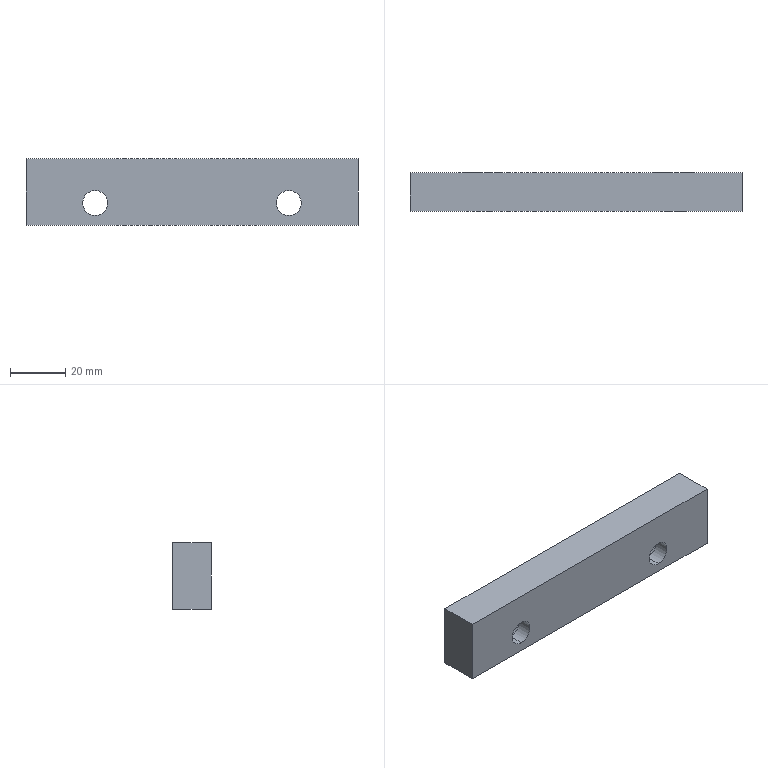Part | STEP file | 1 solid | 16 faces | box 120 x 14 x 24 mm | volume 36593 mm3 | cylinder 8 | plane 8 | commonest cylinder face diameters 9 x4 15 x4
STEP:
#1=CARTESIAN_POINT('',(0.,0.,0.));
#2=DIRECTION('',(0.,0.,1.));
#3=DIRECTION('',(1.,0.,0.));
#4=AXIS2_PLACEMENT_3D('',#1,#2,#3);
#5=CARTESIAN_POINT('',(-35.,5.4,15.5));
#6=VERTEX_POINT('',#5);
#7=CARTESIAN_POINT('',(-35.,14.,15.5));
#8=VERTEX_POINT('',#7);
#9=CARTESIAN_POINT('',(-35.,14.,15.5));
#10=DIRECTION('',(0.,1.,0.));
#11=VECTOR('',#10,1.);
#12=LINE('',#9,#11);
#13=CARTESIAN_POINT('',(-35.,14.,8.));
#14=DIRECTION('',(0.,1.,0.));
#15=DIRECTION('',(0.,0.,1.));
#16=AXIS2_PLACEMENT_3D('',#13,#14,#15);
#17=CYLINDRICAL_SURFACE('',#16,7.5);
#18=CARTESIAN_POINT('',(6.283,0.));
#19=DIRECTION('',(0.,1.));
#20=VECTOR('',#19,1.);
#21=LINE('',#18,#20);
#22=(GEOMETRIC_REPRESENTATION_CONTEXT(2)PARAMETRIC_REPRESENTATION_CONTEXT()REPRESENTATION_CONTEXT('',''));
#23=DEFINITIONAL_REPRESENTATION('',(#21),#22);
#24=PCURVE('',#17,#23);
#25=CARTESIAN_POINT('',(-35.,14.,8.));
#26=DIRECTION('',(0.,1.,0.));
#27=DIRECTION('',(0.,0.,1.));
#28=AXIS2_PLACEMENT_3D('',#25,#26,#27);
#29=CYLINDRICAL_SURFACE('',#28,7.5);
#30=CARTESIAN_POINT('',(0.,0.));
#31=DIRECTION('',(0.,1.));
#32=VECTOR('',#31,1.);
#33=LINE('',#30,#32);
#34=(GEOMETRIC_REPRESENTATION_CONTEXT(2)PARAMETRIC_REPRESENTATION_CONTEXT()REPRESENTATION_CONTEXT('',''));
#35=DEFINITIONAL_REPRESENTATION('',(#33),#34);
#36=PCURVE('',#29,#35);
#37=SURFACE_CURVE('',#12,(#24,#36),.PCURVE_S1.);
#38=EDGE_CURVE('',#6,#8,#37,.T.);
#39=ORIENTED_EDGE('',*,*,#38,.T.);
#40=CARTESIAN_POINT('',(-35.,14.,0.5));
#41=VERTEX_POINT('',#40);
#42=CARTESIAN_POINT('',(-35.,14.,8.));
#43=DIRECTION('',(0.,1.,0.));
#44=DIRECTION('',(0.,0.,1.));
#45=AXIS2_PLACEMENT_3D('',#42,#43,#44);
#46=CIRCLE('',#45,7.5);
#47=CARTESIAN_POINT('',(0.,0.));
#48=DIRECTION('',(1.,0.));
#49=VECTOR('',#48,1.);
#50=LINE('',#47,#49);
#51=(GEOMETRIC_REPRESENTATION_CONTEXT(2)PARAMETRIC_REPRESENTATION_CONTEXT()REPRESENTATION_CONTEXT('',''));
#52=DEFINITIONAL_REPRESENTATION('',(#50),#51);
#53=PCURVE('',#17,#52);
#54=CARTESIAN_POINT('',(0.,14.,0.));
#55=DIRECTION('',(0.,1.,0.));
#56=DIRECTION('',(0.,0.,1.));
#57=AXIS2_PLACEMENT_3D('',#54,#55,#56);
#58=PLANE('',#57);
#59=CARTESIAN_POINT('',(8.,-35.));
#60=DIRECTION('',(1.,0.));
#61=AXIS2_PLACEMENT_2D('',#59,#60);
#62=CIRCLE('',#61,7.5);
#63=(GEOMETRIC_REPRESENTATION_CONTEXT(2)PARAMETRIC_REPRESENTATION_CONTEXT()REPRESENTATION_CONTEXT('',''));
#64=DEFINITIONAL_REPRESENTATION('',(#62),#63);
#65=PCURVE('',#58,#64);
#66=SURFACE_CURVE('',#46,(#53,#65),.PCURVE_S1.);
#67=EDGE_CURVE('',#41,#8,#66,.T.);
#68=ORIENTED_EDGE('',*,*,#67,.F.);
#69=CARTESIAN_POINT('',(-35.,5.4,0.5));
#70=VERTEX_POINT('',#69);
#71=CARTESIAN_POINT('',(-35.,14.,0.5));
#72=DIRECTION('',(0.,1.,0.));
#73=VECTOR('',#72,1.);
#74=LINE('',#71,#73);
#75=CARTESIAN_POINT('',(3.142,0.));
#76=DIRECTION('',(0.,1.));
#77=VECTOR('',#76,1.);
#78=LINE('',#75,#77);
#79=(GEOMETRIC_REPRESENTATION_CONTEXT(2)PARAMETRIC_REPRESENTATION_CONTEXT()REPRESENTATION_CONTEXT('',''));
#80=DEFINITIONAL_REPRESENTATION('',(#78),#79);
#81=PCURVE('',#17,#80);
#82=CARTESIAN_POINT('',(3.142,0.));
#83=DIRECTION('',(0.,1.));
#84=VECTOR('',#83,1.);
#85=LINE('',#82,#84);
#86=(GEOMETRIC_REPRESENTATION_CONTEXT(2)PARAMETRIC_REPRESENTATION_CONTEXT()REPRESENTATION_CONTEXT('',''));
#87=DEFINITIONAL_REPRESENTATION('',(#85),#86);
#88=PCURVE('',#29,#87);
#89=SURFACE_CURVE('',#74,(#81,#88),.PCURVE_S1.);
#90=EDGE_CURVE('',#70,#41,#89,.T.);
#91=ORIENTED_EDGE('',*,*,#90,.F.);
#92=CARTESIAN_POINT('',(-35.,5.4,8.));
#93=DIRECTION('',(0.,1.,0.));
#94=DIRECTION('',(0.,0.,1.));
#95=AXIS2_PLACEMENT_3D('',#92,#93,#94);
#96=CIRCLE('',#95,7.5);
#97=CARTESIAN_POINT('',(0.,-8.6));
#98=DIRECTION('',(1.,0.));
#99=VECTOR('',#98,1.);
#100=LINE('',#97,#99);
#101=(GEOMETRIC_REPRESENTATION_CONTEXT(2)PARAMETRIC_REPRESENTATION_CONTEXT()REPRESENTATION_CONTEXT('',''));
#102=DEFINITIONAL_REPRESENTATION('',(#100),#101);
#103=PCURVE('',#17,#102);
#104=CARTESIAN_POINT('',(-30.5,5.4,8.));
#105=DIRECTION('',(0.,-1.,0.));
#106=DIRECTION('',(0.,0.,-1.));
#107=AXIS2_PLACEMENT_3D('',#104,#105,#106);
#108=PLANE('',#107);
#109=CARTESIAN_POINT('',(-7.5,-4.5));
#110=CARTESIAN_POINT('',(-7.5,8.49));
#111=CARTESIAN_POINT('',(3.75,1.995));
#112=CARTESIAN_POINT('',(15.,-4.5));
#113=CARTESIAN_POINT('',(3.75,-10.995));
#114=CARTESIAN_POINT('',(-7.5,-17.49));
#115=CARTESIAN_POINT('',(-7.5,-4.5));
#116=(BOUNDED_CURVE()B_SPLINE_CURVE(2,(#109,#110,#111,#112,#113,#114,#115),.UNSPECIFIED.,.T.,.F.)B_SPLINE_CURVE_WITH_KNOTS((1,2,2,2,2,1),(-2.094,0.,2.094,4.189,6.283,8.378),.UNSPECIFIED.)CURVE()GEOMETRIC_REPRESENTATION_ITEM()RATIONAL_B_SPLINE_CURVE((1.,0.5,1.,0.5,1.,0.5,1.))REPRESENTATION_ITEM(''));
#117=(GEOMETRIC_REPRESENTATION_CONTEXT(2)PARAMETRIC_REPRESENTATION_CONTEXT()REPRESENTATION_CONTEXT('',''));
#118=DEFINITIONAL_REPRESENTATION('',(#116),#117);
#119=PCURVE('',#108,#118);
#120=SURFACE_CURVE('',#96,(#103,#119),.PCURVE_S1.);
#121=EDGE_CURVE('',#70,#6,#120,.T.);
#122=ORIENTED_EDGE('',*,*,#121,.T.);
#123=EDGE_LOOP('',(#39,#68,#91,#122));
#124=FACE_BOUND('',#123,.F.);
#125=ADVANCED_FACE('',(#124),#17,.F.);
#126=CARTESIAN_POINT('',(-35.,0.,12.5));
#127=VERTEX_POINT('',#126);
#128=CARTESIAN_POINT('',(-35.,5.4,12.5));
#129=VERTEX_POINT('',#128);
#130=CARTESIAN_POINT('',(-35.,14.,12.5));
#131=DIRECTION('',(0.,1.,0.));
#132=VECTOR('',#131,1.);
#133=LINE('',#130,#132);
#134=CARTESIAN_POINT('',(-35.,14.,8.));
#135=DIRECTION('',(0.,1.,0.));
#136=DIRECTION('',(0.,0.,1.));
#137=AXIS2_PLACEMENT_3D('',#134,#135,#136);
#138=CYLINDRICAL_SURFACE('',#137,4.5);
#139=CARTESIAN_POINT('',(6.283,0.));
#140=DIRECTION('',(0.,1.));
#141=VECTOR('',#140,1.);
#142=LINE('',#139,#141);
#143=(GEOMETRIC_REPRESENTATION_CONTEXT(2)PARAMETRIC_REPRESENTATION_CONTEXT()REPRESENTATION_CONTEXT('',''));
#144=DEFINITIONAL_REPRESENTATION('',(#142),#143);
#145=PCURVE('',#138,#144);
#146=CARTESIAN_POINT('',(-35.,14.,8.));
#147=DIRECTION('',(0.,1.,0.));
#148=DIRECTION('',(0.,0.,1.));
#149=AXIS2_PLACEMENT_3D('',#146,#147,#148);
#150=CYLINDRICAL_SURFACE('',#149,4.5);
#151=CARTESIAN_POINT('',(0.,0.));
#152=DIRECTION('',(0.,1.));
#153=VECTOR('',#152,1.);
#154=LINE('',#151,#153);
#155=(GEOMETRIC_REPRESENTATION_CONTEXT(2)PARAMETRIC_REPRESENTATION_CONTEXT()REPRESENTATION_CONTEXT('',''));
#156=DEFINITIONAL_REPRESENTATION('',(#154),#155);
#157=PCURVE('',#150,#156);
#158=SURFACE_CURVE('',#133,(#145,#157),.PCURVE_S1.);
#159=EDGE_CURVE('',#127,#129,#158,.T.);
#160=ORIENTED_EDGE('',*,*,#159,.T.);
#161=CARTESIAN_POINT('',(-35.,5.4,3.5));
#162=VERTEX_POINT('',#161);
#163=CARTESIAN_POINT('',(-35.,5.4,8.));
#164=DIRECTION('',(0.,1.,0.));
#165=DIRECTION('',(0.,0.,1.));
#166=AXIS2_PLACEMENT_3D('',#163,#164,#165);
#167=CIRCLE('',#166,4.5);
#168=CARTESIAN_POINT('',(0.,-8.6));
#169=DIRECTION('',(1.,0.));
#170=VECTOR('',#169,1.);
#171=LINE('',#168,#170);
#172=(GEOMETRIC_REPRESENTATION_CONTEXT(2)PARAMETRIC_REPRESENTATION_CONTEXT()REPRESENTATION_CONTEXT('',''));
#173=DEFINITIONAL_REPRESENTATION('',(#171),#172);
#174=PCURVE('',#138,#173);
#175=CARTESIAN_POINT('',(-4.5,-4.5));
#176=CARTESIAN_POINT('',(-4.5,3.294));
#177=CARTESIAN_POINT('',(2.25,-0.6029));
#178=CARTESIAN_POINT('',(9.,-4.5));
#179=CARTESIAN_POINT('',(2.25,-8.397));
#180=CARTESIAN_POINT('',(-4.5,-12.294));
#181=CARTESIAN_POINT('',(-4.5,-4.5));
#182=(BOUNDED_CURVE()B_SPLINE_CURVE(2,(#175,#176,#177,#178,#179,#180,#181),.UNSPECIFIED.,.T.,.F.)B_SPLINE_CURVE_WITH_KNOTS((1,2,2,2,2,1),(-2.094,0.,2.094,4.189,6.283,8.378),.UNSPECIFIED.)CURVE()GEOMETRIC_REPRESENTATION_ITEM()RATIONAL_B_SPLINE_CURVE((1.,0.5,1.,0.5,1.,0.5,1.))REPRESENTATION_ITEM(''));
#183=(GEOMETRIC_REPRESENTATION_CONTEXT(2)PARAMETRIC_REPRESENTATION_CONTEXT()REPRESENTATION_CONTEXT('',''));
#184=DEFINITIONAL_REPRESENTATION('',(#182),#183);
#185=PCURVE('',#108,#184);
#186=SURFACE_CURVE('',#167,(#174,#185),.PCURVE_S1.);
#187=EDGE_CURVE('',#162,#129,#186,.T.);
#188=ORIENTED_EDGE('',*,*,#187,.F.);
#189=CARTESIAN_POINT('',(-35.,0.,3.5));
#190=VERTEX_POINT('',#189);
#191=CARTESIAN_POINT('',(-35.,14.,3.5));
#192=DIRECTION('',(0.,1.,0.));
#193=VECTOR('',#192,1.);
#194=LINE('',#191,#193);
#195=CARTESIAN_POINT('',(3.142,0.));
#196=DIRECTION('',(0.,1.));
#197=VECTOR('',#196,1.);
#198=LINE('',#195,#197);
#199=(GEOMETRIC_REPRESENTATION_CONTEXT(2)PARAMETRIC_REPRESENTATION_CONTEXT()REPRESENTATION_CONTEXT('',''));
#200=DEFINITIONAL_REPRESENTATION('',(#198),#199);
#201=PCURVE('',#138,#200);
#202=CARTESIAN_POINT('',(3.142,0.));
#203=DIRECTION('',(0.,1.));
#204=VECTOR('',#203,1.);
#205=LINE('',#202,#204);
#206=(GEOMETRIC_REPRESENTATION_CONTEXT(2)PARAMETRIC_REPRESENTATION_CONTEXT()REPRESENTATION_CONTEXT('',''));
#207=DEFINITIONAL_REPRESENTATION('',(#205),#206);
#208=PCURVE('',#150,#207);
#209=SURFACE_CURVE('',#194,(#201,#208),.PCURVE_S1.);
#210=EDGE_CURVE('',#190,#162,#209,.T.);
#211=ORIENTED_EDGE('',*,*,#210,.F.);
#212=CARTESIAN_POINT('',(-35.,0.,8.));
#213=DIRECTION('',(0.,1.,0.));
#214=DIRECTION('',(0.,0.,1.));
#215=AXIS2_PLACEMENT_3D('',#212,#213,#214);
#216=CIRCLE('',#215,4.5);
#217=CARTESIAN_POINT('',(0.,-14.));
#218=DIRECTION('',(1.,0.));
#219=VECTOR('',#218,1.);
#220=LINE('',#217,#219);
#221=(GEOMETRIC_REPRESENTATION_CONTEXT(2)PARAMETRIC_REPRESENTATION_CONTEXT()REPRESENTATION_CONTEXT('',''));
#222=DEFINITIONAL_REPRESENTATION('',(#220),#221);
#223=PCURVE('',#138,#222);
#224=CARTESIAN_POINT('',(0.,0.,0.));
#225=DIRECTION('',(0.,1.,0.));
#226=DIRECTION('',(0.,0.,1.));
#227=AXIS2_PLACEMENT_3D('',#224,#225,#226);
#228=PLANE('',#227);
#229=CARTESIAN_POINT('',(8.,-35.));
#230=DIRECTION('',(1.,0.));
#231=AXIS2_PLACEMENT_2D('',#229,#230);
#232=CIRCLE('',#231,4.5);
#233=(GEOMETRIC_REPRESENTATION_CONTEXT(2)PARAMETRIC_REPRESENTATION_CONTEXT()REPRESENTATION_CONTEXT('',''));
#234=DEFINITIONAL_REPRESENTATION('',(#232),#233);
#235=PCURVE('',#228,#234);
#236=SURFACE_CURVE('',#216,(#223,#235),.PCURVE_S1.);
#237=EDGE_CURVE('',#190,#127,#236,.T.);
#238=ORIENTED_EDGE('',*,*,#237,.T.);
#239=EDGE_LOOP('',(#160,#188,#211,#238));
#240=FACE_BOUND('',#239,.F.);
#241=ADVANCED_FACE('',(#240),#138,.F.);
#242=CARTESIAN_POINT('',(35.,5.4,15.5));
#243=VERTEX_POINT('',#242);
#244=CARTESIAN_POINT('',(35.,14.,15.5));
#245=VERTEX_POINT('',#244);
#246=CARTESIAN_POINT('',(35.,14.,15.5));
#247=DIRECTION('',(0.,1.,0.));
#248=VECTOR('',#247,1.);
#249=LINE('',#246,#248);
#250=CARTESIAN_POINT('',(35.,14.,8.));
#251=DIRECTION('',(0.,1.,0.));
#252=DIRECTION('',(0.,0.,1.));
#253=AXIS2_PLACEMENT_3D('',#250,#251,#252);
#254=CYLINDRICAL_SURFACE('',#253,7.5);
#255=CARTESIAN_POINT('',(6.283,0.));
#256=DIRECTION('',(0.,1.));
#257=VECTOR('',#256,1.);
#258=LINE('',#255,#257);
#259=(GEOMETRIC_REPRESENTATION_CONTEXT(2)PARAMETRIC_REPRESENTATION_CONTEXT()REPRESENTATION_CONTEXT('',''));
#260=DEFINITIONAL_REPRESENTATION('',(#258),#259);
#261=PCURVE('',#254,#260);
#262=CARTESIAN_POINT('',(35.,14.,8.));
#263=DIRECTION('',(0.,1.,0.));
#264=DIRECTION('',(0.,0.,1.));
#265=AXIS2_PLACEMENT_3D('',#262,#263,#264);
#266=CYLINDRICAL_SURFACE('',#265,7.5);
#267=CARTESIAN_POINT('',(0.,0.));
#268=DIRECTION('',(0.,1.));
#269=VECTOR('',#268,1.);
#270=LINE('',#267,#269);
#271=(GEOMETRIC_REPRESENTATION_CONTEXT(2)PARAMETRIC_REPRESENTATION_CONTEXT()REPRESENTATION_CONTEXT('',''));
#272=DEFINITIONAL_REPRESENTATION('',(#270),#271);
#273=PCURVE('',#266,#272);
#274=SURFACE_CURVE('',#249,(#261,#273),.PCURVE_S1.);
#275=EDGE_CURVE('',#243,#245,#274,.T.);
#276=ORIENTED_EDGE('',*,*,#275,.T.);
#277=CARTESIAN_POINT('',(35.,14.,0.5));
#278=VERTEX_POINT('',#277);
#279=CARTESIAN_POINT('',(35.,14.,8.));
#280=DIRECTION('',(0.,1.,0.));
#281=DIRECTION('',(0.,0.,1.));
#282=AXIS2_PLACEMENT_3D('',#279,#280,#281);
#283=CIRCLE('',#282,7.5);
#284=CARTESIAN_POINT('',(0.,0.));
#285=DIRECTION('',(1.,0.));
#286=VECTOR('',#285,1.);
#287=LINE('',#284,#286);
#288=(GEOMETRIC_REPRESENTATION_CONTEXT(2)PARAMETRIC_REPRESENTATION_CONTEXT()REPRESENTATION_CONTEXT('',''));
#289=DEFINITIONAL_REPRESENTATION('',(#287),#288);
#290=PCURVE('',#254,#289);
#291=CARTESIAN_POINT('',(8.,35.));
#292=DIRECTION('',(1.,0.));
#293=AXIS2_PLACEMENT_2D('',#291,#292);
#294=CIRCLE('',#293,7.5);
#295=(GEOMETRIC_REPRESENTATION_CONTEXT(2)PARAMETRIC_REPRESENTATION_CONTEXT()REPRESENTATION_CONTEXT('',''));
#296=DEFINITIONAL_REPRESENTATION('',(#294),#295);
#297=PCURVE('',#58,#296);
#298=SURFACE_CURVE('',#283,(#290,#297),.PCURVE_S1.);
#299=EDGE_CURVE('',#278,#245,#298,.T.);
#300=ORIENTED_EDGE('',*,*,#299,.F.);
#301=CARTESIAN_POINT('',(35.,5.4,0.5));
#302=VERTEX_POINT('',#301);
#303=CARTESIAN_POINT('',(35.,14.,0.5));
#304=DIRECTION('',(0.,1.,0.));
#305=VECTOR('',#304,1.);
#306=LINE('',#303,#305);
#307=CARTESIAN_POINT('',(3.142,0.));
#308=DIRECTION('',(0.,1.));
#309=VECTOR('',#308,1.);
#310=LINE('',#307,#309);
#311=(GEOMETRIC_REPRESENTATION_CONTEXT(2)PARAMETRIC_REPRESENTATION_CONTEXT()REPRESENTATION_CONTEXT('',''));
#312=DEFINITIONAL_REPRESENTATION('',(#310),#311);
#313=PCURVE('',#254,#312);
#314=CARTESIAN_POINT('',(3.142,0.));
#315=DIRECTION('',(0.,1.));
#316=VECTOR('',#315,1.);
#317=LINE('',#314,#316);
#318=(GEOMETRIC_REPRESENTATION_CONTEXT(2)PARAMETRIC_REPRESENTATION_CONTEXT()REPRESENTATION_CONTEXT('',''));
#319=DEFINITIONAL_REPRESENTATION('',(#317),#318);
#320=PCURVE('',#266,#319);
#321=SURFACE_CURVE('',#306,(#313,#320),.PCURVE_S1.);
#322=EDGE_CURVE('',#302,#278,#321,.T.);
#323=ORIENTED_EDGE('',*,*,#322,.F.);
#324=CARTESIAN_POINT('',(35.,5.4,8.));
#325=DIRECTION('',(0.,1.,0.));
#326=DIRECTION('',(0.,0.,1.));
#327=AXIS2_PLACEMENT_3D('',#324,#325,#326);
#328=CIRCLE('',#327,7.5);
#329=CARTESIAN_POINT('',(0.,-8.6));
#330=DIRECTION('',(1.,0.));
#331=VECTOR('',#330,1.);
#332=LINE('',#329,#331);
#333=(GEOMETRIC_REPRESENTATION_CONTEXT(2)PARAMETRIC_REPRESENTATION_CONTEXT()REPRESENTATION_CONTEXT('',''));
#334=DEFINITIONAL_REPRESENTATION('',(#332),#333);
#335=PCURVE('',#254,#334);
#336=CARTESIAN_POINT('',(39.5,5.4,8.));
#337=DIRECTION('',(0.,-1.,0.));
#338=DIRECTION('',(0.,0.,-1.));
#339=AXIS2_PLACEMENT_3D('',#336,#337,#338);
#340=PLANE('',#339);
#341=CARTESIAN_POINT('',(-7.5,-4.5));
#342=CARTESIAN_POINT('',(-7.5,8.49));
#343=CARTESIAN_POINT('',(3.75,1.995));
#344=CARTESIAN_POINT('',(15.,-4.5));
#345=CARTESIAN_POINT('',(3.75,-10.995));
#346=CARTESIAN_POINT('',(-7.5,-17.49));
#347=CARTESIAN_POINT('',(-7.5,-4.5));
#348=(BOUNDED_CURVE()B_SPLINE_CURVE(2,(#341,#342,#343,#344,#345,#346,#347),.UNSPECIFIED.,.T.,.F.)B_SPLINE_CURVE_WITH_KNOTS((1,2,2,2,2,1),(-2.094,0.,2.094,4.189,6.283,8.378),.UNSPECIFIED.)CURVE()GEOMETRIC_REPRESENTATION_ITEM()RATIONAL_B_SPLINE_CURVE((1.,0.5,1.,0.5,1.,0.5,1.))REPRESENTATION_ITEM(''));
#349=(GEOMETRIC_REPRESENTATION_CONTEXT(2)PARAMETRIC_REPRESENTATION_CONTEXT()REPRESENTATION_CONTEXT('',''));
#350=DEFINITIONAL_REPRESENTATION('',(#348),#349);
#351=PCURVE('',#340,#350);
#352=SURFACE_CURVE('',#328,(#335,#351),.PCURVE_S1.);
#353=EDGE_CURVE('',#302,#243,#352,.T.);
#354=ORIENTED_EDGE('',*,*,#353,.T.);
#355=EDGE_LOOP('',(#276,#300,#323,#354));
#356=FACE_BOUND('',#355,.F.);
#357=ADVANCED_FACE('',(#356),#254,.F.);
#358=CARTESIAN_POINT('',(35.,0.,12.5));
#359=VERTEX_POINT('',#358);
#360=CARTESIAN_POINT('',(35.,5.4,12.5));
#361=VERTEX_POINT('',#360);
#362=CARTESIAN_POINT('',(35.,14.,12.5));
#363=DIRECTION('',(0.,1.,0.));
#364=VECTOR('',#363,1.);
#365=LINE('',#362,#364);
#366=CARTESIAN_POINT('',(35.,14.,8.));
#367=DIRECTION('',(0.,1.,0.));
#368=DIRECTION('',(0.,0.,1.));
#369=AXIS2_PLACEMENT_3D('',#366,#367,#368);
#370=CYLINDRICAL_SURFACE('',#369,4.5);
#371=CARTESIAN_POINT('',(6.283,0.));
#372=DIRECTION('',(0.,1.));
#373=VECTOR('',#372,1.);
#374=LINE('',#371,#373);
#375=(GEOMETRIC_REPRESENTATION_CONTEXT(2)PARAMETRIC_REPRESENTATION_CONTEXT()REPRESENTATION_CONTEXT('',''));
#376=DEFINITIONAL_REPRESENTATION('',(#374),#375);
#377=PCURVE('',#370,#376);
#378=CARTESIAN_POINT('',(35.,14.,8.));
#379=DIRECTION('',(0.,1.,0.));
#380=DIRECTION('',(0.,0.,1.));
#381=AXIS2_PLACEMENT_3D('',#378,#379,#380);
#382=CYLINDRICAL_SURFACE('',#381,4.5);
#383=CARTESIAN_POINT('',(0.,0.));
#384=DIRECTION('',(0.,1.));
#385=VECTOR('',#384,1.);
#386=LINE('',#383,#385);
#387=(GEOMETRIC_REPRESENTATION_CONTEXT(2)PARAMETRIC_REPRESENTATION_CONTEXT()REPRESENTATION_CONTEXT('',''));
#388=DEFINITIONAL_REPRESENTATION('',(#386),#387);
#389=PCURVE('',#382,#388);
#390=SURFACE_CURVE('',#365,(#377,#389),.PCURVE_S1.);
#391=EDGE_CURVE('',#359,#361,#390,.T.);
#392=ORIENTED_EDGE('',*,*,#391,.T.);
#393=CARTESIAN_POINT('',(35.,5.4,3.5));
#394=VERTEX_POINT('',#393);
#395=CARTESIAN_POINT('',(35.,5.4,8.));
#396=DIRECTION('',(0.,1.,0.));
#397=DIRECTION('',(0.,0.,1.));
#398=AXIS2_PLACEMENT_3D('',#395,#396,#397);
#399=CIRCLE('',#398,4.5);
#400=CARTESIAN_POINT('',(0.,-8.6));
#401=DIRECTION('',(1.,0.));
#402=VECTOR('',#401,1.);
#403=LINE('',#400,#402);
#404=(GEOMETRIC_REPRESENTATION_CONTEXT(2)PARAMETRIC_REPRESENTATION_CONTEXT()REPRESENTATION_CONTEXT('',''));
#405=DEFINITIONAL_REPRESENTATION('',(#403),#404);
#406=PCURVE('',#370,#405);
#407=CARTESIAN_POINT('',(-4.5,-4.5));
#408=CARTESIAN_POINT('',(-4.5,3.294));
#409=CARTESIAN_POINT('',(2.25,-0.6029));
#410=CARTESIAN_POINT('',(9.,-4.5));
#411=CARTESIAN_POINT('',(2.25,-8.397));
#412=CARTESIAN_POINT('',(-4.5,-12.294));
#413=CARTESIAN_POINT('',(-4.5,-4.5));
#414=(BOUNDED_CURVE()B_SPLINE_CURVE(2,(#407,#408,#409,#410,#411,#412,#413),.UNSPECIFIED.,.T.,.F.)B_SPLINE_CURVE_WITH_KNOTS((1,2,2,2,2,1),(-2.094,0.,2.094,4.189,6.283,8.378),.UNSPECIFIED.)CURVE()GEOMETRIC_REPRESENTATION_ITEM()RATIONAL_B_SPLINE_CURVE((1.,0.5,1.,0.5,1.,0.5,1.))REPRESENTATION_ITEM(''));
#415=(GEOMETRIC_REPRESENTATION_CONTEXT(2)PARAMETRIC_REPRESENTATION_CONTEXT()REPRESENTATION_CONTEXT('',''));
#416=DEFINITIONAL_REPRESENTATION('',(#414),#415);
#417=PCURVE('',#340,#416);
#418=SURFACE_CURVE('',#399,(#406,#417),.PCURVE_S1.);
#419=EDGE_CURVE('',#394,#361,#418,.T.);
#420=ORIENTED_EDGE('',*,*,#419,.F.);
#421=CARTESIAN_POINT('',(35.,0.,3.5));
#422=VERTEX_POINT('',#421);
#423=CARTESIAN_POINT('',(35.,14.,3.5));
#424=DIRECTION('',(0.,1.,0.));
#425=VECTOR('',#424,1.);
#426=LINE('',#423,#425);
#427=CARTESIAN_POINT('',(3.142,0.));
#428=DIRECTION('',(0.,1.));
#429=VECTOR('',#428,1.);
#430=LINE('',#427,#429);
#431=(GEOMETRIC_REPRESENTATION_CONTEXT(2)PARAMETRIC_REPRESENTATION_CONTEXT()REPRESENTATION_CONTEXT('',''));
#432=DEFINITIONAL_REPRESENTATION('',(#430),#431);
#433=PCURVE('',#370,#432);
#434=CARTESIAN_POINT('',(3.142,0.));
#435=DIRECTION('',(0.,1.));
#436=VECTOR('',#435,1.);
#437=LINE('',#434,#436);
#438=(GEOMETRIC_REPRESENTATION_CONTEXT(2)PARAMETRIC_REPRESENTATION_CONTEXT()REPRESENTATION_CONTEXT('',''));
#439=DEFINITIONAL_REPRESENTATION('',(#437),#438);
#440=PCURVE('',#382,#439);
#441=SURFACE_CURVE('',#426,(#433,#440),.PCURVE_S1.);
#442=EDGE_CURVE('',#422,#394,#441,.T.);
#443=ORIENTED_EDGE('',*,*,#442,.F.);
#444=CARTESIAN_POINT('',(35.,0.,8.));
#445=DIRECTION('',(0.,1.,0.));
#446=DIRECTION('',(0.,0.,1.));
#447=AXIS2_PLACEMENT_3D('',#444,#445,#446);
#448=CIRCLE('',#447,4.5);
#449=CARTESIAN_POINT('',(0.,-14.));
#450=DIRECTION('',(1.,0.));
#451=VECTOR('',#450,1.);
#452=LINE('',#449,#451);
#453=(GEOMETRIC_REPRESENTATION_CONTEXT(2)PARAMETRIC_REPRESENTATION_CONTEXT()REPRESENTATION_CONTEXT('',''));
#454=DEFINITIONAL_REPRESENTATION('',(#452),#453);
#455=PCURVE('',#370,#454);
#456=CARTESIAN_POINT('',(8.,35.));
#457=DIRECTION('',(1.,0.));
#458=AXIS2_PLACEMENT_2D('',#456,#457);
#459=CIRCLE('',#458,4.5);
#460=(GEOMETRIC_REPRESENTATION_CONTEXT(2)PARAMETRIC_REPRESENTATION_CONTEXT()REPRESENTATION_CONTEXT('',''));
#461=DEFINITIONAL_REPRESENTATION('',(#459),#460);
#462=PCURVE('',#228,#461);
#463=SURFACE_CURVE('',#448,(#455,#462),.PCURVE_S1.);
#464=EDGE_CURVE('',#422,#359,#463,.T.);
#465=ORIENTED_EDGE('',*,*,#464,.T.);
#466=EDGE_LOOP('',(#392,#420,#443,#465));
#467=FACE_BOUND('',#466,.F.);
#468=ADVANCED_FACE('',(#467),#370,.F.);
#469=CARTESIAN_POINT('',(-60.,0.,0.));
#470=VERTEX_POINT('',#469);
#471=CARTESIAN_POINT('',(-60.,0.,24.));
#472=VERTEX_POINT('',#471);
#473=CARTESIAN_POINT('',(-60.,0.,0.));
#474=DIRECTION('',(0.,0.,1.));
#475=VECTOR('',#474,1.);
#476=LINE('',#473,#475);
#477=CARTESIAN_POINT('',(-60.,14.,0.));
#478=DIRECTION('',(1.,0.,0.));
#479=DIRECTION('',(0.,0.,-1.));
#480=AXIS2_PLACEMENT_3D('',#477,#478,#479);
#481=PLANE('',#480);
#482=CARTESIAN_POINT('',(0.,-14.));
#483=DIRECTION('',(-1.,0.));
#484=VECTOR('',#483,1.);
#485=LINE('',#482,#484);
#486=(GEOMETRIC_REPRESENTATION_CONTEXT(2)PARAMETRIC_REPRESENTATION_CONTEXT()REPRESENTATION_CONTEXT('',''));
#487=DEFINITIONAL_REPRESENTATION('',(#485),#486);
#488=PCURVE('',#481,#487);
#489=CARTESIAN_POINT('',(0.,-60.));
#490=DIRECTION('',(1.,0.));
#491=VECTOR('',#490,1.);
#492=LINE('',#489,#491);
#493=(GEOMETRIC_REPRESENTATION_CONTEXT(2)PARAMETRIC_REPRESENTATION_CONTEXT()REPRESENTATION_CONTEXT('',''));
#494=DEFINITIONAL_REPRESENTATION('',(#492),#493);
#495=PCURVE('',#228,#494);
#496=SURFACE_CURVE('',#476,(#488,#495),.PCURVE_S1.);
#497=EDGE_CURVE('',#470,#472,#496,.T.);
#498=ORIENTED_EDGE('',*,*,#497,.T.);
#499=CARTESIAN_POINT('',(-60.,14.,24.));
#500=VERTEX_POINT('',#499);
#501=CARTESIAN_POINT('',(-60.,14.,24.));
#502=DIRECTION('',(0.,-1.,0.));
#503=VECTOR('',#502,1.);
#504=LINE('',#501,#503);
#505=CARTESIAN_POINT('',(-24.,0.));
#506=DIRECTION('',(0.,-1.));
#507=VECTOR('',#506,1.);
#508=LINE('',#505,#507);
#509=(GEOMETRIC_REPRESENTATION_CONTEXT(2)PARAMETRIC_REPRESENTATION_CONTEXT()REPRESENTATION_CONTEXT('',''));
#510=DEFINITIONAL_REPRESENTATION('',(#508),#509);
#511=PCURVE('',#481,#510);
#512=CARTESIAN_POINT('',(-60.,14.,24.));
#513=DIRECTION('',(0.,0.,-1.));
#514=DIRECTION('',(-1.,0.,0.));
#515=AXIS2_PLACEMENT_3D('',#512,#513,#514);
#516=PLANE('',#515);
#517=CARTESIAN_POINT('',(0.,0.));
#518=DIRECTION('',(0.,-1.));
#519=VECTOR('',#518,1.);
#520=LINE('',#517,#519);
#521=(GEOMETRIC_REPRESENTATION_CONTEXT(2)PARAMETRIC_REPRESENTATION_CONTEXT()REPRESENTATION_CONTEXT('',''));
#522=DEFINITIONAL_REPRESENTATION('',(#520),#521);
#523=PCURVE('',#516,#522);
#524=SURFACE_CURVE('',#504,(#511,#523),.PCURVE_S1.);
#525=EDGE_CURVE('',#500,#472,#524,.T.);
#526=ORIENTED_EDGE('',*,*,#525,.F.);
#527=CARTESIAN_POINT('',(-60.,14.,0.));
#528=VERTEX_POINT('',#527);
#529=CARTESIAN_POINT('',(-60.,14.,0.));
#530=DIRECTION('',(0.,0.,1.));
#531=VECTOR('',#530,1.);
#532=LINE('',#529,#531);
#533=CARTESIAN_POINT('',(0.,0.));
#534=DIRECTION('',(-1.,0.));
#535=VECTOR('',#534,1.);
#536=LINE('',#533,#535);
#537=(GEOMETRIC_REPRESENTATION_CONTEXT(2)PARAMETRIC_REPRESENTATION_CONTEXT()REPRESENTATION_CONTEXT('',''));
#538=DEFINITIONAL_REPRESENTATION('',(#536),#537);
#539=PCURVE('',#481,#538);
#540=CARTESIAN_POINT('',(0.,-60.));
#541=DIRECTION('',(1.,0.));
#542=VECTOR('',#541,1.);
#543=LINE('',#540,#542);
#544=(GEOMETRIC_REPRESENTATION_CONTEXT(2)PARAMETRIC_REPRESENTATION_CONTEXT()REPRESENTATION_CONTEXT('',''));
#545=DEFINITIONAL_REPRESENTATION('',(#543),#544);
#546=PCURVE('',#58,#545);
#547=SURFACE_CURVE('',#532,(#539,#546),.PCURVE_S1.);
#548=EDGE_CURVE('',#528,#500,#547,.T.);
#549=ORIENTED_EDGE('',*,*,#548,.F.);
#550=CARTESIAN_POINT('',(-60.,14.,0.));
#551=DIRECTION('',(0.,-1.,0.));
#552=VECTOR('',#551,1.);
#553=LINE('',#550,#552);
#554=CARTESIAN_POINT('',(0.,0.));
#555=DIRECTION('',(0.,-1.));
#556=VECTOR('',#555,1.);
#557=LINE('',#554,#556);
#558=(GEOMETRIC_REPRESENTATION_CONTEXT(2)PARAMETRIC_REPRESENTATION_CONTEXT()REPRESENTATION_CONTEXT('',''));
#559=DEFINITIONAL_REPRESENTATION('',(#557),#558);
#560=PCURVE('',#481,#559);
#561=CARTESIAN_POINT('',(-60.,14.,0.));
#562=DIRECTION('',(0.,0.,1.));
#563=DIRECTION('',(1.,0.,0.));
#564=AXIS2_PLACEMENT_3D('',#561,#562,#563);
#565=PLANE('',#564);
#566=CARTESIAN_POINT('',(0.,0.));
#567=DIRECTION('',(0.,-1.));
#568=VECTOR('',#567,1.);
#569=LINE('',#566,#568);
#570=(GEOMETRIC_REPRESENTATION_CONTEXT(2)PARAMETRIC_REPRESENTATION_CONTEXT()REPRESENTATION_CONTEXT('',''));
#571=DEFINITIONAL_REPRESENTATION('',(#569),#570);
#572=PCURVE('',#565,#571);
#573=SURFACE_CURVE('',#553,(#560,#572),.PCURVE_S1.);
#574=EDGE_CURVE('',#528,#470,#573,.T.);
#575=ORIENTED_EDGE('',*,*,#574,.T.);
#576=EDGE_LOOP('',(#498,#526,#549,#575));
#577=FACE_BOUND('',#576,.T.);
#578=ADVANCED_FACE('',(#577),#481,.F.);
#579=CARTESIAN_POINT('',(60.,0.,24.));
#580=VERTEX_POINT('',#579);
#581=CARTESIAN_POINT('',(-60.,0.,24.));
#582=DIRECTION('',(1.,0.,0.));
#583=VECTOR('',#582,1.);
#584=LINE('',#581,#583);
#585=CARTESIAN_POINT('',(0.,-14.));
#586=DIRECTION('',(-1.,0.));
#587=VECTOR('',#586,1.);
#588=LINE('',#585,#587);
#589=(GEOMETRIC_REPRESENTATION_CONTEXT(2)PARAMETRIC_REPRESENTATION_CONTEXT()REPRESENTATION_CONTEXT('',''));
#590=DEFINITIONAL_REPRESENTATION('',(#588),#589);
#591=PCURVE('',#516,#590);
#592=CARTESIAN_POINT('',(24.,-60.));
#593=DIRECTION('',(0.,1.));
#594=VECTOR('',#593,1.);
#595=LINE('',#592,#594);
#596=(GEOMETRIC_REPRESENTATION_CONTEXT(2)PARAMETRIC_REPRESENTATION_CONTEXT()REPRESENTATION_CONTEXT('',''));
#597=DEFINITIONAL_REPRESENTATION('',(#595),#596);
#598=PCURVE('',#228,#597);
#599=SURFACE_CURVE('',#584,(#591,#598),.PCURVE_S1.);
#600=EDGE_CURVE('',#472,#580,#599,.T.);
#601=ORIENTED_EDGE('',*,*,#600,.T.);
#602=CARTESIAN_POINT('',(60.,14.,24.));
#603=VERTEX_POINT('',#602);
#604=CARTESIAN_POINT('',(60.,14.,24.));
#605=DIRECTION('',(0.,-1.,0.));
#606=VECTOR('',#605,1.);
#607=LINE('',#604,#606);
#608=CARTESIAN_POINT('',(-120.,0.));
#609=DIRECTION('',(0.,-1.));
#610=VECTOR('',#609,1.);
#611=LINE('',#608,#610);
#612=(GEOMETRIC_REPRESENTATION_CONTEXT(2)PARAMETRIC_REPRESENTATION_CONTEXT()REPRESENTATION_CONTEXT('',''));
#613=DEFINITIONAL_REPRESENTATION('',(#611),#612);
#614=PCURVE('',#516,#613);
#615=CARTESIAN_POINT('',(60.,14.,0.));
#616=DIRECTION('',(-1.,0.,0.));
#617=DIRECTION('',(0.,0.,1.));
#618=AXIS2_PLACEMENT_3D('',#615,#616,#617);
#619=PLANE('',#618);
#620=CARTESIAN_POINT('',(24.,0.));
#621=DIRECTION('',(0.,-1.));
#622=VECTOR('',#621,1.);
#623=LINE('',#620,#622);
#624=(GEOMETRIC_REPRESENTATION_CONTEXT(2)PARAMETRIC_REPRESENTATION_CONTEXT()REPRESENTATION_CONTEXT('',''));
#625=DEFINITIONAL_REPRESENTATION('',(#623),#624);
#626=PCURVE('',#619,#625);
#627=SURFACE_CURVE('',#607,(#614,#626),.PCURVE_S1.);
#628=EDGE_CURVE('',#603,#580,#627,.T.);
#629=ORIENTED_EDGE('',*,*,#628,.F.);
#630=CARTESIAN_POINT('',(-60.,14.,24.));
#631=DIRECTION('',(1.,0.,0.));
#632=VECTOR('',#631,1.);
#633=LINE('',#630,#632);
#634=CARTESIAN_POINT('',(0.,0.));
#635=DIRECTION('',(-1.,0.));
#636=VECTOR('',#635,1.);
#637=LINE('',#634,#636);
#638=(GEOMETRIC_REPRESENTATION_CONTEXT(2)PARAMETRIC_REPRESENTATION_CONTEXT()REPRESENTATION_CONTEXT('',''));
#639=DEFINITIONAL_REPRESENTATION('',(#637),#638);
#640=PCURVE('',#516,#639);
#641=CARTESIAN_POINT('',(24.,-60.));
#642=DIRECTION('',(0.,1.));
#643=VECTOR('',#642,1.);
#644=LINE('',#641,#643);
#645=(GEOMETRIC_REPRESENTATION_CONTEXT(2)PARAMETRIC_REPRESENTATION_CONTEXT()REPRESENTATION_CONTEXT('',''));
#646=DEFINITIONAL_REPRESENTATION('',(#644),#645);
#647=PCURVE('',#58,#646);
#648=SURFACE_CURVE('',#633,(#640,#647),.PCURVE_S1.);
#649=EDGE_CURVE('',#500,#603,#648,.T.);
#650=ORIENTED_EDGE('',*,*,#649,.F.);
#651=ORIENTED_EDGE('',*,*,#525,.T.);
#652=EDGE_LOOP('',(#601,#629,#650,#651));
#653=FACE_BOUND('',#652,.T.);
#654=ADVANCED_FACE('',(#653),#516,.F.);
#655=CARTESIAN_POINT('',(60.,0.,0.));
#656=VERTEX_POINT('',#655);
#657=CARTESIAN_POINT('',(60.,0.,0.));
#658=DIRECTION('',(0.,0.,-1.));
#659=VECTOR('',#658,1.);
#660=LINE('',#657,#659);
#661=CARTESIAN_POINT('',(0.,-14.));
#662=DIRECTION('',(-1.,0.));
#663=VECTOR('',#662,1.);
#664=LINE('',#661,#663);
#665=(GEOMETRIC_REPRESENTATION_CONTEXT(2)PARAMETRIC_REPRESENTATION_CONTEXT()REPRESENTATION_CONTEXT('',''));
#666=DEFINITIONAL_REPRESENTATION('',(#664),#665);
#667=PCURVE('',#619,#666);
#668=CARTESIAN_POINT('',(0.,60.));
#669=DIRECTION('',(-1.,0.));
#670=VECTOR('',#669,1.);
#671=LINE('',#668,#670);
#672=(GEOMETRIC_REPRESENTATION_CONTEXT(2)PARAMETRIC_REPRESENTATION_CONTEXT()REPRESENTATION_CONTEXT('',''));
#673=DEFINITIONAL_REPRESENTATION('',(#671),#672);
#674=PCURVE('',#228,#673);
#675=SURFACE_CURVE('',#660,(#667,#674),.PCURVE_S1.);
#676=EDGE_CURVE('',#580,#656,#675,.T.);
#677=ORIENTED_EDGE('',*,*,#676,.T.);
#678=CARTESIAN_POINT('',(60.,14.,0.));
#679=VERTEX_POINT('',#678);
#680=CARTESIAN_POINT('',(60.,14.,0.));
#681=DIRECTION('',(0.,-1.,0.));
#682=VECTOR('',#681,1.);
#683=LINE('',#680,#682);
#684=CARTESIAN_POINT('',(0.,0.));
#685=DIRECTION('',(0.,-1.));
#686=VECTOR('',#685,1.);
#687=LINE('',#684,#686);
#688=(GEOMETRIC_REPRESENTATION_CONTEXT(2)PARAMETRIC_REPRESENTATION_CONTEXT()REPRESENTATION_CONTEXT('',''));
#689=DEFINITIONAL_REPRESENTATION('',(#687),#688);
#690=PCURVE('',#619,#689);
#691=CARTESIAN_POINT('',(120.,0.));
#692=DIRECTION('',(0.,-1.));
#693=VECTOR('',#692,1.);
#694=LINE('',#691,#693);
#695=(GEOMETRIC_REPRESENTATION_CONTEXT(2)PARAMETRIC_REPRESENTATION_CONTEXT()REPRESENTATION_CONTEXT('',''));
#696=DEFINITIONAL_REPRESENTATION('',(#694),#695);
#697=PCURVE('',#565,#696);
#698=SURFACE_CURVE('',#683,(#690,#697),.PCURVE_S1.);
#699=EDGE_CURVE('',#679,#656,#698,.T.);
#700=ORIENTED_EDGE('',*,*,#699,.F.);
#701=CARTESIAN_POINT('',(60.,14.,0.));
#702=DIRECTION('',(0.,0.,-1.));
#703=VECTOR('',#702,1.);
#704=LINE('',#701,#703);
#705=CARTESIAN_POINT('',(0.,0.));
#706=DIRECTION('',(-1.,0.));
#707=VECTOR('',#706,1.);
#708=LINE('',#705,#707);
#709=(GEOMETRIC_REPRESENTATION_CONTEXT(2)PARAMETRIC_REPRESENTATION_CONTEXT()REPRESENTATION_CONTEXT('',''));
#710=DEFINITIONAL_REPRESENTATION('',(#708),#709);
#711=PCURVE('',#619,#710);
#712=CARTESIAN_POINT('',(0.,60.));
#713=DIRECTION('',(-1.,0.));
#714=VECTOR('',#713,1.);
#715=LINE('',#712,#714);
#716=(GEOMETRIC_REPRESENTATION_CONTEXT(2)PARAMETRIC_REPRESENTATION_CONTEXT()REPRESENTATION_CONTEXT('',''));
#717=DEFINITIONAL_REPRESENTATION('',(#715),#716);
#718=PCURVE('',#58,#717);
#719=SURFACE_CURVE('',#704,(#711,#718),.PCURVE_S1.);
#720=EDGE_CURVE('',#603,#679,#719,.T.);
#721=ORIENTED_EDGE('',*,*,#720,.F.);
#722=ORIENTED_EDGE('',*,*,#628,.T.);
#723=EDGE_LOOP('',(#677,#700,#721,#722));
#724=FACE_BOUND('',#723,.T.);
#725=ADVANCED_FACE('',(#724),#619,.F.);
#726=CARTESIAN_POINT('',(-60.,0.,0.));
#727=DIRECTION('',(-1.,0.,0.));
#728=VECTOR('',#727,1.);
#729=LINE('',#726,#728);
#730=CARTESIAN_POINT('',(0.,-14.));
#731=DIRECTION('',(-1.,0.));
#732=VECTOR('',#731,1.);
#733=LINE('',#730,#732);
#734=(GEOMETRIC_REPRESENTATION_CONTEXT(2)PARAMETRIC_REPRESENTATION_CONTEXT()REPRESENTATION_CONTEXT('',''));
#735=DEFINITIONAL_REPRESENTATION('',(#733),#734);
#736=PCURVE('',#565,#735);
#737=CARTESIAN_POINT('',(0.,-60.));
#738=DIRECTION('',(0.,-1.));
#739=VECTOR('',#738,1.);
#740=LINE('',#737,#739);
#741=(GEOMETRIC_REPRESENTATION_CONTEXT(2)PARAMETRIC_REPRESENTATION_CONTEXT()REPRESENTATION_CONTEXT('',''));
#742=DEFINITIONAL_REPRESENTATION('',(#740),#741);
#743=PCURVE('',#228,#742);
#744=SURFACE_CURVE('',#729,(#736,#743),.PCURVE_S1.);
#745=EDGE_CURVE('',#656,#470,#744,.T.);
#746=ORIENTED_EDGE('',*,*,#745,.T.);
#747=ORIENTED_EDGE('',*,*,#574,.F.);
#748=CARTESIAN_POINT('',(-60.,14.,0.));
#749=DIRECTION('',(-1.,0.,0.));
#750=VECTOR('',#749,1.);
#751=LINE('',#748,#750);
#752=CARTESIAN_POINT('',(0.,0.));
#753=DIRECTION('',(-1.,0.));
#754=VECTOR('',#753,1.);
#755=LINE('',#752,#754);
#756=(GEOMETRIC_REPRESENTATION_CONTEXT(2)PARAMETRIC_REPRESENTATION_CONTEXT()REPRESENTATION_CONTEXT('',''));
#757=DEFINITIONAL_REPRESENTATION('',(#755),#756);
#758=PCURVE('',#565,#757);
#759=CARTESIAN_POINT('',(0.,-60.));
#760=DIRECTION('',(0.,-1.));
#761=VECTOR('',#760,1.);
#762=LINE('',#759,#761);
#763=(GEOMETRIC_REPRESENTATION_CONTEXT(2)PARAMETRIC_REPRESENTATION_CONTEXT()REPRESENTATION_CONTEXT('',''));
#764=DEFINITIONAL_REPRESENTATION('',(#762),#763);
#765=PCURVE('',#58,#764);
#766=SURFACE_CURVE('',#751,(#758,#765),.PCURVE_S1.);
#767=EDGE_CURVE('',#679,#528,#766,.T.);
#768=ORIENTED_EDGE('',*,*,#767,.F.);
#769=ORIENTED_EDGE('',*,*,#699,.T.);
#770=EDGE_LOOP('',(#746,#747,#768,#769));
#771=FACE_BOUND('',#770,.T.);
#772=ADVANCED_FACE('',(#771),#565,.F.);
#773=CARTESIAN_POINT('',(-35.,14.,8.));
#774=DIRECTION('',(0.,1.,0.));
#775=DIRECTION('',(0.,0.,1.));
#776=AXIS2_PLACEMENT_3D('',#773,#774,#775);
#777=CIRCLE('',#776,7.5);
#778=CARTESIAN_POINT('',(8.,-35.));
#779=DIRECTION('',(1.,0.));
#780=AXIS2_PLACEMENT_2D('',#778,#779);
#781=CIRCLE('',#780,7.5);
#782=(GEOMETRIC_REPRESENTATION_CONTEXT(2)PARAMETRIC_REPRESENTATION_CONTEXT()REPRESENTATION_CONTEXT('',''));
#783=DEFINITIONAL_REPRESENTATION('',(#781),#782);
#784=PCURVE('',#58,#783);
#785=CARTESIAN_POINT('',(0.,0.));
#786=DIRECTION('',(1.,0.));
#787=VECTOR('',#786,1.);
#788=LINE('',#785,#787);
#789=(GEOMETRIC_REPRESENTATION_CONTEXT(2)PARAMETRIC_REPRESENTATION_CONTEXT()REPRESENTATION_CONTEXT('',''));
#790=DEFINITIONAL_REPRESENTATION('',(#788),#789);
#791=PCURVE('',#29,#790);
#792=SURFACE_CURVE('',#777,(#784,#791),.PCURVE_S1.);
#793=EDGE_CURVE('',#8,#41,#792,.T.);
#794=ORIENTED_EDGE('',*,*,#793,.F.);
#795=ORIENTED_EDGE('',*,*,#67,.F.);
#796=EDGE_LOOP('',(#794,#795));
#797=FACE_BOUND('',#796,.T.);
#798=CARTESIAN_POINT('',(35.,14.,8.));
#799=DIRECTION('',(0.,1.,0.));
#800=DIRECTION('',(0.,0.,1.));
#801=AXIS2_PLACEMENT_3D('',#798,#799,#800);
#802=CIRCLE('',#801,7.5);
#803=CARTESIAN_POINT('',(8.,35.));
#804=DIRECTION('',(1.,0.));
#805=AXIS2_PLACEMENT_2D('',#803,#804);
#806=CIRCLE('',#805,7.5);
#807=(GEOMETRIC_REPRESENTATION_CONTEXT(2)PARAMETRIC_REPRESENTATION_CONTEXT()REPRESENTATION_CONTEXT('',''));
#808=DEFINITIONAL_REPRESENTATION('',(#806),#807);
#809=PCURVE('',#58,#808);
#810=CARTESIAN_POINT('',(0.,0.));
#811=DIRECTION('',(1.,0.));
#812=VECTOR('',#811,1.);
#813=LINE('',#810,#812);
#814=(GEOMETRIC_REPRESENTATION_CONTEXT(2)PARAMETRIC_REPRESENTATION_CONTEXT()REPRESENTATION_CONTEXT('',''));
#815=DEFINITIONAL_REPRESENTATION('',(#813),#814);
#816=PCURVE('',#266,#815);
#817=SURFACE_CURVE('',#802,(#809,#816),.PCURVE_S1.);
#818=EDGE_CURVE('',#245,#278,#817,.T.);
#819=ORIENTED_EDGE('',*,*,#818,.F.);
#820=ORIENTED_EDGE('',*,*,#299,.F.);
#821=EDGE_LOOP('',(#819,#820));
#822=FACE_BOUND('',#821,.T.);
#823=ORIENTED_EDGE('',*,*,#548,.T.);
#824=ORIENTED_EDGE('',*,*,#649,.T.);
#825=ORIENTED_EDGE('',*,*,#720,.T.);
#826=ORIENTED_EDGE('',*,*,#767,.T.);
#827=EDGE_LOOP('',(#823,#824,#825,#826));
#828=FACE_BOUND('',#827,.T.);
#829=ADVANCED_FACE('',(#797,#822,#828),#58,.T.);
#830=CARTESIAN_POINT('',(-35.,0.,8.));
#831=DIRECTION('',(0.,1.,0.));
#832=DIRECTION('',(0.,0.,1.));
#833=AXIS2_PLACEMENT_3D('',#830,#831,#832);
#834=CIRCLE('',#833,4.5);
#835=CARTESIAN_POINT('',(8.,-35.));
#836=DIRECTION('',(1.,0.));
#837=AXIS2_PLACEMENT_2D('',#835,#836);
#838=CIRCLE('',#837,4.5);
#839=(GEOMETRIC_REPRESENTATION_CONTEXT(2)PARAMETRIC_REPRESENTATION_CONTEXT()REPRESENTATION_CONTEXT('',''));
#840=DEFINITIONAL_REPRESENTATION('',(#838),#839);
#841=PCURVE('',#228,#840);
#842=CARTESIAN_POINT('',(0.,-14.));
#843=DIRECTION('',(1.,0.));
#844=VECTOR('',#843,1.);
#845=LINE('',#842,#844);
#846=(GEOMETRIC_REPRESENTATION_CONTEXT(2)PARAMETRIC_REPRESENTATION_CONTEXT()REPRESENTATION_CONTEXT('',''));
#847=DEFINITIONAL_REPRESENTATION('',(#845),#846);
#848=PCURVE('',#150,#847);
#849=SURFACE_CURVE('',#834,(#841,#848),.PCURVE_S1.);
#850=EDGE_CURVE('',#127,#190,#849,.T.);
#851=ORIENTED_EDGE('',*,*,#850,.T.);
#852=ORIENTED_EDGE('',*,*,#237,.T.);
#853=EDGE_LOOP('',(#851,#852));
#854=FACE_BOUND('',#853,.T.);
#855=CARTESIAN_POINT('',(35.,0.,8.));
#856=DIRECTION('',(0.,1.,0.));
#857=DIRECTION('',(0.,0.,1.));
#858=AXIS2_PLACEMENT_3D('',#855,#856,#857);
#859=CIRCLE('',#858,4.5);
#860=CARTESIAN_POINT('',(8.,35.));
#861=DIRECTION('',(1.,0.));
#862=AXIS2_PLACEMENT_2D('',#860,#861);
#863=CIRCLE('',#862,4.5);
#864=(GEOMETRIC_REPRESENTATION_CONTEXT(2)PARAMETRIC_REPRESENTATION_CONTEXT()REPRESENTATION_CONTEXT('',''));
#865=DEFINITIONAL_REPRESENTATION('',(#863),#864);
#866=PCURVE('',#228,#865);
#867=CARTESIAN_POINT('',(0.,-14.));
#868=DIRECTION('',(1.,0.));
#869=VECTOR('',#868,1.);
#870=LINE('',#867,#869);
#871=(GEOMETRIC_REPRESENTATION_CONTEXT(2)PARAMETRIC_REPRESENTATION_CONTEXT()REPRESENTATION_CONTEXT('',''));
#872=DEFINITIONAL_REPRESENTATION('',(#870),#871);
#873=PCURVE('',#382,#872);
#874=SURFACE_CURVE('',#859,(#866,#873),.PCURVE_S1.);
#875=EDGE_CURVE('',#359,#422,#874,.T.);
#876=ORIENTED_EDGE('',*,*,#875,.T.);
#877=ORIENTED_EDGE('',*,*,#464,.T.);
#878=EDGE_LOOP('',(#876,#877));
#879=FACE_BOUND('',#878,.T.);
#880=ORIENTED_EDGE('',*,*,#497,.F.);
#881=ORIENTED_EDGE('',*,*,#745,.F.);
#882=ORIENTED_EDGE('',*,*,#676,.F.);
#883=ORIENTED_EDGE('',*,*,#600,.F.);
#884=EDGE_LOOP('',(#880,#881,#882,#883));
#885=FACE_BOUND('',#884,.T.);
#886=ADVANCED_FACE('',(#854,#879,#885),#228,.F.);
#887=CARTESIAN_POINT('',(35.,5.4,8.));
#888=DIRECTION('',(0.,1.,0.));
#889=DIRECTION('',(0.,0.,1.));
#890=AXIS2_PLACEMENT_3D('',#887,#888,#889);
#891=CIRCLE('',#890,4.5);
#892=CARTESIAN_POINT('',(0.,-8.6));
#893=DIRECTION('',(1.,0.));
#894=VECTOR('',#893,1.);
#895=LINE('',#892,#894);
#896=(GEOMETRIC_REPRESENTATION_CONTEXT(2)PARAMETRIC_REPRESENTATION_CONTEXT()REPRESENTATION_CONTEXT('',''));
#897=DEFINITIONAL_REPRESENTATION('',(#895),#896);
#898=PCURVE('',#382,#897);
#899=CARTESIAN_POINT('',(-4.5,-4.5));
#900=CARTESIAN_POINT('',(-4.5,3.294));
#901=CARTESIAN_POINT('',(2.25,-0.6029));
#902=CARTESIAN_POINT('',(9.,-4.5));
#903=CARTESIAN_POINT('',(2.25,-8.397));
#904=CARTESIAN_POINT('',(-4.5,-12.294));
#905=CARTESIAN_POINT('',(-4.5,-4.5));
#906=(BOUNDED_CURVE()B_SPLINE_CURVE(2,(#899,#900,#901,#902,#903,#904,#905),.UNSPECIFIED.,.T.,.F.)B_SPLINE_CURVE_WITH_KNOTS((1,2,2,2,2,1),(-2.094,0.,2.094,4.189,6.283,8.378),.UNSPECIFIED.)CURVE()GEOMETRIC_REPRESENTATION_ITEM()RATIONAL_B_SPLINE_CURVE((1.,0.5,1.,0.5,1.,0.5,1.))REPRESENTATION_ITEM(''));
#907=(GEOMETRIC_REPRESENTATION_CONTEXT(2)PARAMETRIC_REPRESENTATION_CONTEXT()REPRESENTATION_CONTEXT('',''));
#908=DEFINITIONAL_REPRESENTATION('',(#906),#907);
#909=PCURVE('',#340,#908);
#910=SURFACE_CURVE('',#891,(#898,#909),.PCURVE_S1.);
#911=EDGE_CURVE('',#361,#394,#910,.T.);
#912=ORIENTED_EDGE('',*,*,#911,.F.);
#913=ORIENTED_EDGE('',*,*,#391,.F.);
#914=ORIENTED_EDGE('',*,*,#875,.T.);
#915=ORIENTED_EDGE('',*,*,#442,.T.);
#916=EDGE_LOOP('',(#912,#913,#914,#915));
#917=FACE_BOUND('',#916,.F.);
#918=ADVANCED_FACE('',(#917),#382,.F.);
#919=ORIENTED_EDGE('',*,*,#911,.F.);
#920=ORIENTED_EDGE('',*,*,#419,.F.);
#921=EDGE_LOOP('',(#919,#920));
#922=FACE_BOUND('',#921,.T.);
#923=CARTESIAN_POINT('',(35.,5.4,8.));
#924=DIRECTION('',(0.,1.,0.));
#925=DIRECTION('',(0.,0.,1.));
#926=AXIS2_PLACEMENT_3D('',#923,#924,#925);
#927=CIRCLE('',#926,7.5);
#928=CARTESIAN_POINT('',(-7.5,-4.5));
#929=CARTESIAN_POINT('',(-7.5,8.49));
#930=CARTESIAN_POINT('',(3.75,1.995));
#931=CARTESIAN_POINT('',(15.,-4.5));
#932=CARTESIAN_POINT('',(3.75,-10.995));
#933=CARTESIAN_POINT('',(-7.5,-17.49));
#934=CARTESIAN_POINT('',(-7.5,-4.5));
#935=(BOUNDED_CURVE()B_SPLINE_CURVE(2,(#928,#929,#930,#931,#932,#933,#934),.UNSPECIFIED.,.T.,.F.)B_SPLINE_CURVE_WITH_KNOTS((1,2,2,2,2,1),(-2.094,0.,2.094,4.189,6.283,8.378),.UNSPECIFIED.)CURVE()GEOMETRIC_REPRESENTATION_ITEM()RATIONAL_B_SPLINE_CURVE((1.,0.5,1.,0.5,1.,0.5,1.))REPRESENTATION_ITEM(''));
#936=(GEOMETRIC_REPRESENTATION_CONTEXT(2)PARAMETRIC_REPRESENTATION_CONTEXT()REPRESENTATION_CONTEXT('',''));
#937=DEFINITIONAL_REPRESENTATION('',(#935),#936);
#938=PCURVE('',#340,#937);
#939=CARTESIAN_POINT('',(0.,-8.6));
#940=DIRECTION('',(1.,0.));
#941=VECTOR('',#940,1.);
#942=LINE('',#939,#941);
#943=(GEOMETRIC_REPRESENTATION_CONTEXT(2)PARAMETRIC_REPRESENTATION_CONTEXT()REPRESENTATION_CONTEXT('',''));
#944=DEFINITIONAL_REPRESENTATION('',(#942),#943);
#945=PCURVE('',#266,#944);
#946=SURFACE_CURVE('',#927,(#938,#945),.PCURVE_S1.);
#947=EDGE_CURVE('',#243,#302,#946,.T.);
#948=ORIENTED_EDGE('',*,*,#947,.T.);
#949=ORIENTED_EDGE('',*,*,#353,.T.);
#950=EDGE_LOOP('',(#948,#949));
#951=FACE_BOUND('',#950,.T.);
#952=ADVANCED_FACE('',(#922,#951),#340,.F.);
#953=ORIENTED_EDGE('',*,*,#818,.F.);
#954=ORIENTED_EDGE('',*,*,#275,.F.);
#955=ORIENTED_EDGE('',*,*,#947,.T.);
#956=ORIENTED_EDGE('',*,*,#322,.T.);
#957=EDGE_LOOP('',(#953,#954,#955,#956));
#958=FACE_BOUND('',#957,.F.);
#959=ADVANCED_FACE('',(#958),#266,.F.);
#960=CARTESIAN_POINT('',(-35.,5.4,8.));
#961=DIRECTION('',(0.,1.,0.));
#962=DIRECTION('',(0.,0.,1.));
#963=AXIS2_PLACEMENT_3D('',#960,#961,#962);
#964=CIRCLE('',#963,4.5);
#965=CARTESIAN_POINT('',(0.,-8.6));
#966=DIRECTION('',(1.,0.));
#967=VECTOR('',#966,1.);
#968=LINE('',#965,#967);
#969=(GEOMETRIC_REPRESENTATION_CONTEXT(2)PARAMETRIC_REPRESENTATION_CONTEXT()REPRESENTATION_CONTEXT('',''));
#970=DEFINITIONAL_REPRESENTATION('',(#968),#969);
#971=PCURVE('',#150,#970);
#972=CARTESIAN_POINT('',(-4.5,-4.5));
#973=CARTESIAN_POINT('',(-4.5,3.294));
#974=CARTESIAN_POINT('',(2.25,-0.6029));
#975=CARTESIAN_POINT('',(9.,-4.5));
#976=CARTESIAN_POINT('',(2.25,-8.397));
#977=CARTESIAN_POINT('',(-4.5,-12.294));
#978=CARTESIAN_POINT('',(-4.5,-4.5));
#979=(BOUNDED_CURVE()B_SPLINE_CURVE(2,(#972,#973,#974,#975,#976,#977,#978),.UNSPECIFIED.,.T.,.F.)B_SPLINE_CURVE_WITH_KNOTS((1,2,2,2,2,1),(-2.094,0.,2.094,4.189,6.283,8.378),.UNSPECIFIED.)CURVE()GEOMETRIC_REPRESENTATION_ITEM()RATIONAL_B_SPLINE_CURVE((1.,0.5,1.,0.5,1.,0.5,1.))REPRESENTATION_ITEM(''));
#980=(GEOMETRIC_REPRESENTATION_CONTEXT(2)PARAMETRIC_REPRESENTATION_CONTEXT()REPRESENTATION_CONTEXT('',''));
#981=DEFINITIONAL_REPRESENTATION('',(#979),#980);
#982=PCURVE('',#108,#981);
#983=SURFACE_CURVE('',#964,(#971,#982),.PCURVE_S1.);
#984=EDGE_CURVE('',#129,#162,#983,.T.);
#985=ORIENTED_EDGE('',*,*,#984,.F.);
#986=ORIENTED_EDGE('',*,*,#159,.F.);
#987=ORIENTED_EDGE('',*,*,#850,.T.);
#988=ORIENTED_EDGE('',*,*,#210,.T.);
#989=EDGE_LOOP('',(#985,#986,#987,#988));
#990=FACE_BOUND('',#989,.F.);
#991=ADVANCED_FACE('',(#990),#150,.F.);
#992=ORIENTED_EDGE('',*,*,#984,.F.);
#993=ORIENTED_EDGE('',*,*,#187,.F.);
#994=EDGE_LOOP('',(#992,#993));
#995=FACE_BOUND('',#994,.T.);
#996=CARTESIAN_POINT('',(-35.,5.4,8.));
#997=DIRECTION('',(0.,1.,0.));
#998=DIRECTION('',(0.,0.,1.));
#999=AXIS2_PLACEMENT_3D('',#996,#997,#998);
#1000=CIRCLE('',#999,7.5);
#1001=CARTESIAN_POINT('',(-7.5,-4.5));
#1002=CARTESIAN_POINT('',(-7.5,8.49));
#1003=CARTESIAN_POINT('',(3.75,1.995));
#1004=CARTESIAN_POINT('',(15.,-4.5));
#1005=CARTESIAN_POINT('',(3.75,-10.995));
#1006=CARTESIAN_POINT('',(-7.5,-17.49));
#1007=CARTESIAN_POINT('',(-7.5,-4.5));
#1008=(BOUNDED_CURVE()B_SPLINE_CURVE(2,(#1001,#1002,#1003,#1004,#1005,#1006,#1007),.UNSPECIFIED.,.T.,.F.)B_SPLINE_CURVE_WITH_KNOTS((1,2,2,2,2,1),(-2.094,0.,2.094,4.189,6.283,8.378),.UNSPECIFIED.)CURVE()GEOMETRIC_REPRESENTATION_ITEM()RATIONAL_B_SPLINE_CURVE((1.,0.5,1.,0.5,1.,0.5,1.))REPRESENTATION_ITEM(''));
#1009=(GEOMETRIC_REPRESENTATION_CONTEXT(2)PARAMETRIC_REPRESENTATION_CONTEXT()REPRESENTATION_CONTEXT('',''));
#1010=DEFINITIONAL_REPRESENTATION('',(#1008),#1009);
#1011=PCURVE('',#108,#1010);
#1012=CARTESIAN_POINT('',(0.,-8.6));
#1013=DIRECTION('',(1.,0.));
#1014=VECTOR('',#1013,1.);
#1015=LINE('',#1012,#1014);
#1016=(GEOMETRIC_REPRESENTATION_CONTEXT(2)PARAMETRIC_REPRESENTATION_CONTEXT()REPRESENTATION_CONTEXT('',''));
#1017=DEFINITIONAL_REPRESENTATION('',(#1015),#1016);
#1018=PCURVE('',#29,#1017);
#1019=SURFACE_CURVE('',#1000,(#1011,#1018),.PCURVE_S1.);
#1020=EDGE_CURVE('',#6,#70,#1019,.T.);
#1021=ORIENTED_EDGE('',*,*,#1020,.T.);
#1022=ORIENTED_EDGE('',*,*,#121,.T.);
#1023=EDGE_LOOP('',(#1021,#1022));
#1024=FACE_BOUND('',#1023,.T.);
#1025=ADVANCED_FACE('',(#995,#1024),#108,.F.);
#1026=ORIENTED_EDGE('',*,*,#793,.F.);
#1027=ORIENTED_EDGE('',*,*,#38,.F.);
#1028=ORIENTED_EDGE('',*,*,#1020,.T.);
#1029=ORIENTED_EDGE('',*,*,#90,.T.);
#1030=EDGE_LOOP('',(#1026,#1027,#1028,#1029));
#1031=FACE_BOUND('',#1030,.F.);
#1032=ADVANCED_FACE('',(#1031),#29,.F.);
#1033=CLOSED_SHELL('',(#125,#241,#357,#468,#578,#654,#725,#772,#829,#886,#918,#952,#959,#991,#1025,#1032));
#1034=MANIFOLD_SOLID_BREP('',#1033);
#1035=(LENGTH_UNIT()NAMED_UNIT(*)SI_UNIT(.MILLI.,.METRE.));
#1036=UNCERTAINTY_MEASURE_WITH_UNIT(LENGTH_MEASURE(0.0000001),#1035,'','');
#1037=(NAMED_UNIT(*)PLANE_ANGLE_UNIT()SI_UNIT($,.RADIAN.));
#1038=(NAMED_UNIT(*)SI_UNIT($,.STERADIAN.)SOLID_ANGLE_UNIT());
#1039=(GEOMETRIC_REPRESENTATION_CONTEXT(3)GLOBAL_UNCERTAINTY_ASSIGNED_CONTEXT((#1036))GLOBAL_UNIT_ASSIGNED_CONTEXT((#1035,#1037,#1038))REPRESENTATION_CONTEXT('',''));
#1040=ADVANCED_BREP_SHAPE_REPRESENTATION('',(#4,#1034),#1039);